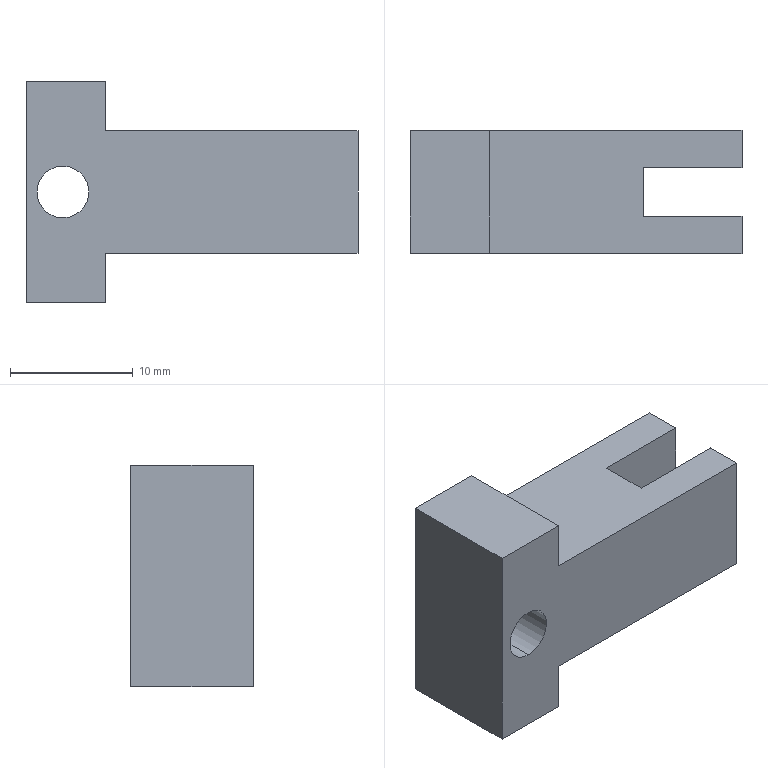Part | SolidWorks | features ICE 7, Extrusion 1, HoleWzd 1, MirrorPattern 1 | 1 solid | 26 faces | box 27 x 10 x 18 mm | volume 2677 mm3 | plane 20 | cylinder 6 | commonest cylinder face diameters 2 x2 2.6 x2 4.2 x2
STEP:
#1=CARTESIAN_POINT('',(-16.,10.,-2.1));
#2=VERTEX_POINT('',#1);
#3=CARTESIAN_POINT('',(-16.,10.,2.1));
#4=VERTEX_POINT('',#3);
#5=CARTESIAN_POINT('',(-16.,10.,0.));
#6=DIRECTION('',(0.,1.,0.));
#7=DIRECTION('',(0.,0.,1.));
#8=AXIS2_PLACEMENT_3D('',#5,#6,#7);
#9=CIRCLE('',#8,2.1);
#10=EDGE_CURVE('',#2,#4,#9,.T.);
#11=ORIENTED_EDGE('',*,*,#10,.T.);
#12=CARTESIAN_POINT('',(-16.,0.,2.1));
#13=VERTEX_POINT('',#12);
#14=CARTESIAN_POINT('',(-16.,0.,2.1));
#15=DIRECTION('',(0.,-1.,0.));
#16=VECTOR('',#15,1000.);
#17=LINE('',#14,#16);
#18=EDGE_CURVE('',#4,#13,#17,.T.);
#19=ORIENTED_EDGE('',*,*,#18,.T.);
#20=CARTESIAN_POINT('',(-16.,0.,-2.1));
#21=VERTEX_POINT('',#20);
#22=CARTESIAN_POINT('',(-16.,0.,0.));
#23=DIRECTION('',(0.,-1.,0.));
#24=DIRECTION('',(0.,0.,-1.));
#25=AXIS2_PLACEMENT_3D('',#22,#23,#24);
#26=CIRCLE('',#25,2.1);
#27=EDGE_CURVE('',#13,#21,#26,.T.);
#28=ORIENTED_EDGE('',*,*,#27,.T.);
#29=CARTESIAN_POINT('',(-16.,0.,-2.1));
#30=DIRECTION('',(0.,-1.,0.));
#31=VECTOR('',#30,1000.);
#32=LINE('',#29,#31);
#33=EDGE_CURVE('',#2,#21,#32,.T.);
#34=ORIENTED_EDGE('',*,*,#33,.F.);
#35=EDGE_LOOP('',(#11,#19,#28,#34));
#36=FACE_OUTER_BOUND('',#35,.T.);
#37=CARTESIAN_POINT('',(-16.,0.,0.));
#38=DIRECTION('',(0.,-1.,0.));
#39=DIRECTION('',(0.,0.,-1.));
#40=AXIS2_PLACEMENT_3D('',#37,#38,#39);
#41=CYLINDRICAL_SURFACE('',#40,2.1);
#42=ADVANCED_FACE('',(#36),#41,.F.);
#43=CARTESIAN_POINT('',(-2.,5.,-1.3));
#44=VERTEX_POINT('',#43);
#45=CARTESIAN_POINT('',(-2.,5.,1.3));
#46=VERTEX_POINT('',#45);
#47=CARTESIAN_POINT('',(-2.,5.,0.));
#48=DIRECTION('',(1.,0.,0.));
#49=DIRECTION('',(0.,0.,-1.));
#50=AXIS2_PLACEMENT_3D('',#47,#48,#49);
#51=CIRCLE('',#50,1.3);
#52=EDGE_CURVE('',#44,#46,#51,.T.);
#53=ORIENTED_EDGE('',*,*,#52,.T.);
#54=CARTESIAN_POINT('',(-1.,5.,1.3));
#55=VERTEX_POINT('',#54);
#56=CARTESIAN_POINT('',(-2.,5.,1.3));
#57=DIRECTION('',(1.,0.,0.));
#58=VECTOR('',#57,1000.);
#59=LINE('',#56,#58);
#60=EDGE_CURVE('',#46,#55,#59,.T.);
#61=ORIENTED_EDGE('',*,*,#60,.T.);
#62=CARTESIAN_POINT('',(-1.,5.,-1.3));
#63=VERTEX_POINT('',#62);
#64=CARTESIAN_POINT('',(-1.,5.,0.));
#65=DIRECTION('',(1.,0.,0.));
#66=DIRECTION('',(0.,0.,-1.));
#67=AXIS2_PLACEMENT_3D('',#64,#65,#66);
#68=CIRCLE('',#67,1.3);
#69=EDGE_CURVE('',#63,#55,#68,.T.);
#70=ORIENTED_EDGE('',*,*,#69,.F.);
#71=CARTESIAN_POINT('',(-2.,5.,-1.3));
#72=DIRECTION('',(1.,0.,0.));
#73=VECTOR('',#72,1000.);
#74=LINE('',#71,#73);
#75=EDGE_CURVE('',#44,#63,#74,.T.);
#76=ORIENTED_EDGE('',*,*,#75,.F.);
#77=EDGE_LOOP('',(#53,#61,#70,#76));
#78=FACE_OUTER_BOUND('',#77,.T.);
#79=CARTESIAN_POINT('',(-2.,5.,0.));
#80=DIRECTION('',(1.,0.,0.));
#81=DIRECTION('',(0.,0.,-1.));
#82=AXIS2_PLACEMENT_3D('',#79,#80,#81);
#83=CYLINDRICAL_SURFACE('',#82,1.3);
#84=ADVANCED_FACE('',(#78),#83,.T.);
#85=CARTESIAN_POINT('',(-2.,5.,-1.));
#86=VERTEX_POINT('',#85);
#87=CARTESIAN_POINT('',(-2.,5.,1.));
#88=VERTEX_POINT('',#87);
#89=CARTESIAN_POINT('',(-2.,5.,0.));
#90=DIRECTION('',(1.,0.,0.));
#91=DIRECTION('',(0.,0.,-1.));
#92=AXIS2_PLACEMENT_3D('',#89,#90,#91);
#93=CIRCLE('',#92,1.);
#94=EDGE_CURVE('',#86,#88,#93,.T.);
#95=ORIENTED_EDGE('',*,*,#94,.F.);
#96=CARTESIAN_POINT('',(-4.,5.,-1.));
#97=VERTEX_POINT('',#96);
#98=CARTESIAN_POINT('',(-1.,5.,-1.));
#99=DIRECTION('',(-1.,0.,0.));
#100=VECTOR('',#99,1000.);
#101=LINE('',#98,#100);
#102=EDGE_CURVE('',#86,#97,#101,.T.);
#103=ORIENTED_EDGE('',*,*,#102,.T.);
#104=CARTESIAN_POINT('',(-4.,5.,1.));
#105=VERTEX_POINT('',#104);
#106=CARTESIAN_POINT('',(-4.,5.,0.));
#107=DIRECTION('',(1.,0.,0.));
#108=DIRECTION('',(0.,0.,-1.));
#109=AXIS2_PLACEMENT_3D('',#106,#107,#108);
#110=CIRCLE('',#109,1.);
#111=EDGE_CURVE('',#97,#105,#110,.T.);
#112=ORIENTED_EDGE('',*,*,#111,.T.);
#113=CARTESIAN_POINT('',(-1.,5.,1.));
#114=DIRECTION('',(-1.,0.,0.));
#115=VECTOR('',#114,1000.);
#116=LINE('',#113,#115);
#117=EDGE_CURVE('',#88,#105,#116,.T.);
#118=ORIENTED_EDGE('',*,*,#117,.F.);
#119=EDGE_LOOP('',(#95,#103,#112,#118));
#120=FACE_OUTER_BOUND('',#119,.T.);
#121=CARTESIAN_POINT('',(-1.,5.,0.));
#122=DIRECTION('',(-1.,0.,0.));
#123=DIRECTION('',(0.,0.,1.));
#124=AXIS2_PLACEMENT_3D('',#121,#122,#123);
#125=CYLINDRICAL_SURFACE('',#124,1.);
#126=ADVANCED_FACE('',(#120),#125,.T.);
#127=ORIENTED_EDGE('',*,*,#102,.F.);
#128=CARTESIAN_POINT('',(-2.,5.,0.));
#129=DIRECTION('',(1.,0.,0.));
#130=DIRECTION('',(0.,0.,-1.));
#131=AXIS2_PLACEMENT_3D('',#128,#129,#130);
#132=CIRCLE('',#131,1.);
#133=EDGE_CURVE('',#88,#86,#132,.T.);
#134=ORIENTED_EDGE('',*,*,#133,.F.);
#135=ORIENTED_EDGE('',*,*,#117,.T.);
#136=CARTESIAN_POINT('',(-4.,5.,0.));
#137=DIRECTION('',(1.,0.,0.));
#138=DIRECTION('',(0.,0.,-1.));
#139=AXIS2_PLACEMENT_3D('',#136,#137,#138);
#140=CIRCLE('',#139,1.);
#141=EDGE_CURVE('',#105,#97,#140,.T.);
#142=ORIENTED_EDGE('',*,*,#141,.T.);
#143=EDGE_LOOP('',(#127,#134,#135,#142));
#144=FACE_OUTER_BOUND('',#143,.T.);
#145=CARTESIAN_POINT('',(-1.,5.,0.));
#146=DIRECTION('',(-1.,0.,0.));
#147=DIRECTION('',(0.,0.,1.));
#148=AXIS2_PLACEMENT_3D('',#145,#146,#147);
#149=CYLINDRICAL_SURFACE('',#148,1.);
#150=ADVANCED_FACE('',(#144),#149,.T.);
#151=CARTESIAN_POINT('',(0.,3.,5.));
#152=VERTEX_POINT('',#151);
#153=CARTESIAN_POINT('',(0.,3.,3.));
#154=VERTEX_POINT('',#153);
#155=CARTESIAN_POINT('',(0.,3.,5.));
#156=DIRECTION('',(0.,0.,-1.));
#157=VECTOR('',#156,1000.);
#158=LINE('',#155,#157);
#159=EDGE_CURVE('',#152,#154,#158,.T.);
#160=ORIENTED_EDGE('',*,*,#159,.T.);
#161=CARTESIAN_POINT('',(0.,7.,3.));
#162=VERTEX_POINT('',#161);
#163=CARTESIAN_POINT('',(0.,3.,3.));
#164=DIRECTION('',(0.,-1.,0.));
#165=VECTOR('',#164,1000.);
#166=LINE('',#163,#165);
#167=EDGE_CURVE('',#162,#154,#166,.T.);
#168=ORIENTED_EDGE('',*,*,#167,.F.);
#169=CARTESIAN_POINT('',(0.,7.,5.));
#170=VERTEX_POINT('',#169);
#171=CARTESIAN_POINT('',(0.,7.,5.));
#172=DIRECTION('',(0.,0.,-1.));
#173=VECTOR('',#172,1000.);
#174=LINE('',#171,#173);
#175=EDGE_CURVE('',#170,#162,#174,.T.);
#176=ORIENTED_EDGE('',*,*,#175,.F.);
#177=CARTESIAN_POINT('',(0.,3.,5.));
#178=DIRECTION('',(0.,1.,0.));
#179=VECTOR('',#178,1000.);
#180=LINE('',#177,#179);
#181=EDGE_CURVE('',#152,#170,#180,.T.);
#182=ORIENTED_EDGE('',*,*,#181,.F.);
#183=EDGE_LOOP('',(#160,#168,#176,#182));
#184=FACE_OUTER_BOUND('',#183,.T.);
#185=CARTESIAN_POINT('',(0.,3.,5.));
#186=DIRECTION('',(-1.,0.,0.));
#187=DIRECTION('',(0.,0.,1.));
#188=AXIS2_PLACEMENT_3D('',#185,#186,#187);
#189=PLANE('',#188);
#190=ADVANCED_FACE('',(#184),#189,.F.);
#191=CARTESIAN_POINT('',(-12.5,10.,-5.));
#192=VERTEX_POINT('',#191);
#193=CARTESIAN_POINT('',(-12.5,0.,-5.));
#194=VERTEX_POINT('',#193);
#195=CARTESIAN_POINT('',(-12.5,0.,-5.));
#196=DIRECTION('',(0.,-1.,0.));
#197=VECTOR('',#196,1000.);
#198=LINE('',#195,#197);
#199=EDGE_CURVE('',#192,#194,#198,.T.);
#200=ORIENTED_EDGE('',*,*,#199,.F.);
#201=CARTESIAN_POINT('',(8.,10.,-5.));
#202=VERTEX_POINT('',#201);
#203=CARTESIAN_POINT('',(8.,10.,-5.));
#204=DIRECTION('',(-1.,0.,0.));
#205=VECTOR('',#204,1000.);
#206=LINE('',#203,#205);
#207=EDGE_CURVE('',#202,#192,#206,.T.);
#208=ORIENTED_EDGE('',*,*,#207,.F.);
#209=CARTESIAN_POINT('',(8.,7.,-5.));
#210=VERTEX_POINT('',#209);
#211=CARTESIAN_POINT('',(8.,10.,-5.));
#212=DIRECTION('',(0.,-1.,0.));
#213=VECTOR('',#212,1000.);
#214=LINE('',#211,#213);
#215=EDGE_CURVE('',#202,#210,#214,.T.);
#216=ORIENTED_EDGE('',*,*,#215,.T.);
#217=CARTESIAN_POINT('',(0.,7.,-5.));
#218=VERTEX_POINT('',#217);
#219=CARTESIAN_POINT('',(16.,7.,-5.));
#220=DIRECTION('',(1.,0.,0.));
#221=VECTOR('',#220,1000.);
#222=LINE('',#219,#221);
#223=EDGE_CURVE('',#218,#210,#222,.T.);
#224=ORIENTED_EDGE('',*,*,#223,.F.);
#225=CARTESIAN_POINT('',(0.,3.,-5.));
#226=VERTEX_POINT('',#225);
#227=CARTESIAN_POINT('',(0.,3.,-5.));
#228=DIRECTION('',(0.,1.,0.));
#229=VECTOR('',#228,1000.);
#230=LINE('',#227,#229);
#231=EDGE_CURVE('',#226,#218,#230,.T.);
#232=ORIENTED_EDGE('',*,*,#231,.F.);
#233=CARTESIAN_POINT('',(8.,3.,-5.));
#234=VERTEX_POINT('',#233);
#235=CARTESIAN_POINT('',(8.,3.,-5.));
#236=DIRECTION('',(1.,0.,0.));
#237=VECTOR('',#236,1000.);
#238=LINE('',#235,#237);
#239=EDGE_CURVE('',#226,#234,#238,.T.);
#240=ORIENTED_EDGE('',*,*,#239,.T.);
#241=CARTESIAN_POINT('',(8.,0.,-5.));
#242=VERTEX_POINT('',#241);
#243=CARTESIAN_POINT('',(8.,10.,-5.));
#244=DIRECTION('',(0.,-1.,0.));
#245=VECTOR('',#244,1000.);
#246=LINE('',#243,#245);
#247=EDGE_CURVE('',#234,#242,#246,.T.);
#248=ORIENTED_EDGE('',*,*,#247,.T.);
#249=CARTESIAN_POINT('',(8.,0.,-5.));
#250=DIRECTION('',(-1.,0.,0.));
#251=VECTOR('',#250,1000.);
#252=LINE('',#249,#251);
#253=EDGE_CURVE('',#242,#194,#252,.T.);
#254=ORIENTED_EDGE('',*,*,#253,.T.);
#255=EDGE_LOOP('',(#200,#208,#216,#224,#232,#240,#248,#254));
#256=FACE_OUTER_BOUND('',#255,.T.);
#257=CARTESIAN_POINT('',(8.,10.,-5.));
#258=DIRECTION('',(0.,0.,1.));
#259=DIRECTION('',(1.,0.,0.));
#260=AXIS2_PLACEMENT_3D('',#257,#258,#259);
#261=PLANE('',#260);
#262=ADVANCED_FACE('',(#256),#261,.F.);
#263=ORIENTED_EDGE('',*,*,#247,.F.);
#264=CARTESIAN_POINT('',(8.,3.,5.));
#265=VERTEX_POINT('',#264);
#266=CARTESIAN_POINT('',(8.,3.,5.));
#267=DIRECTION('',(0.,0.,1.));
#268=VECTOR('',#267,1000.);
#269=LINE('',#266,#268);
#270=EDGE_CURVE('',#234,#265,#269,.T.);
#271=ORIENTED_EDGE('',*,*,#270,.T.);
#272=CARTESIAN_POINT('',(8.,0.,5.));
#273=VERTEX_POINT('',#272);
#274=CARTESIAN_POINT('',(8.,10.,5.));
#275=DIRECTION('',(0.,-1.,0.));
#276=VECTOR('',#275,1000.);
#277=LINE('',#274,#276);
#278=EDGE_CURVE('',#265,#273,#277,.T.);
#279=ORIENTED_EDGE('',*,*,#278,.T.);
#280=CARTESIAN_POINT('',(8.,0.,5.));
#281=DIRECTION('',(0.,0.,-1.));
#282=VECTOR('',#281,1000.);
#283=LINE('',#280,#282);
#284=EDGE_CURVE('',#273,#242,#283,.T.);
#285=ORIENTED_EDGE('',*,*,#284,.T.);
#286=EDGE_LOOP('',(#263,#271,#279,#285));
#287=FACE_OUTER_BOUND('',#286,.T.);
#288=CARTESIAN_POINT('',(8.,10.,5.));
#289=DIRECTION('',(-1.,0.,0.));
#290=DIRECTION('',(0.,0.,1.));
#291=AXIS2_PLACEMENT_3D('',#288,#289,#290);
#292=PLANE('',#291);
#293=ADVANCED_FACE('',(#287),#292,.F.);
#294=CARTESIAN_POINT('',(-12.5,10.,5.));
#295=VERTEX_POINT('',#294);
#296=CARTESIAN_POINT('',(8.,10.,5.));
#297=VERTEX_POINT('',#296);
#298=CARTESIAN_POINT('',(8.,10.,5.));
#299=DIRECTION('',(1.,0.,0.));
#300=VECTOR('',#299,1000.);
#301=LINE('',#298,#300);
#302=EDGE_CURVE('',#295,#297,#301,.T.);
#303=ORIENTED_EDGE('',*,*,#302,.F.);
#304=CARTESIAN_POINT('',(-12.5,0.,5.));
#305=VERTEX_POINT('',#304);
#306=CARTESIAN_POINT('',(-12.5,0.,5.));
#307=DIRECTION('',(0.,-1.,0.));
#308=VECTOR('',#307,1000.);
#309=LINE('',#306,#308);
#310=EDGE_CURVE('',#295,#305,#309,.T.);
#311=ORIENTED_EDGE('',*,*,#310,.T.);
#312=CARTESIAN_POINT('',(8.,0.,5.));
#313=DIRECTION('',(1.,0.,0.));
#314=VECTOR('',#313,1000.);
#315=LINE('',#312,#314);
#316=EDGE_CURVE('',#305,#273,#315,.T.);
#317=ORIENTED_EDGE('',*,*,#316,.T.);
#318=ORIENTED_EDGE('',*,*,#278,.F.);
#319=CARTESIAN_POINT('',(16.,3.,5.));
#320=DIRECTION('',(-1.,0.,0.));
#321=VECTOR('',#320,1000.);
#322=LINE('',#319,#321);
#323=EDGE_CURVE('',#265,#152,#322,.T.);
#324=ORIENTED_EDGE('',*,*,#323,.T.);
#325=ORIENTED_EDGE('',*,*,#181,.T.);
#326=CARTESIAN_POINT('',(8.,7.,5.));
#327=VERTEX_POINT('',#326);
#328=CARTESIAN_POINT('',(16.,7.,5.));
#329=DIRECTION('',(1.,0.,0.));
#330=VECTOR('',#329,1000.);
#331=LINE('',#328,#330);
#332=EDGE_CURVE('',#170,#327,#331,.T.);
#333=ORIENTED_EDGE('',*,*,#332,.T.);
#334=CARTESIAN_POINT('',(8.,10.,5.));
#335=DIRECTION('',(0.,-1.,0.));
#336=VECTOR('',#335,1000.);
#337=LINE('',#334,#336);
#338=EDGE_CURVE('',#297,#327,#337,.T.);
#339=ORIENTED_EDGE('',*,*,#338,.F.);
#340=EDGE_LOOP('',(#303,#311,#317,#318,#324,#325,#333,#339));
#341=FACE_OUTER_BOUND('',#340,.T.);
#342=CARTESIAN_POINT('',(8.,10.,5.));
#343=DIRECTION('',(0.,0.,-1.));
#344=DIRECTION('',(-1.,0.,0.));
#345=AXIS2_PLACEMENT_3D('',#342,#343,#344);
#346=PLANE('',#345);
#347=ADVANCED_FACE('',(#341),#346,.F.);
#348=ORIENTED_EDGE('',*,*,#338,.T.);
#349=CARTESIAN_POINT('',(8.,7.,5.));
#350=DIRECTION('',(0.,0.,-1.));
#351=VECTOR('',#350,1000.);
#352=LINE('',#349,#351);
#353=EDGE_CURVE('',#327,#210,#352,.T.);
#354=ORIENTED_EDGE('',*,*,#353,.T.);
#355=ORIENTED_EDGE('',*,*,#215,.F.);
#356=CARTESIAN_POINT('',(8.,10.,5.));
#357=DIRECTION('',(0.,0.,-1.));
#358=VECTOR('',#357,1000.);
#359=LINE('',#356,#358);
#360=EDGE_CURVE('',#297,#202,#359,.T.);
#361=ORIENTED_EDGE('',*,*,#360,.F.);
#362=EDGE_LOOP('',(#348,#354,#355,#361));
#363=FACE_OUTER_BOUND('',#362,.T.);
#364=CARTESIAN_POINT('',(8.,10.,5.));
#365=DIRECTION('',(-1.,0.,0.));
#366=DIRECTION('',(0.,0.,1.));
#367=AXIS2_PLACEMENT_3D('',#364,#365,#366);
#368=PLANE('',#367);
#369=ADVANCED_FACE('',(#363),#368,.F.);
#370=ORIENTED_EDGE('',*,*,#10,.F.);
#371=CARTESIAN_POINT('',(-16.,10.,0.));
#372=DIRECTION('',(0.,1.,0.));
#373=DIRECTION('',(0.,0.,1.));
#374=AXIS2_PLACEMENT_3D('',#371,#372,#373);
#375=CIRCLE('',#374,2.1);
#376=EDGE_CURVE('',#4,#2,#375,.T.);
#377=ORIENTED_EDGE('',*,*,#376,.F.);
#378=EDGE_LOOP('',(#370,#377));
#379=FACE_BOUND('',#378,.T.);
#380=ORIENTED_EDGE('',*,*,#207,.T.);
#381=CARTESIAN_POINT('',(-12.5,10.,-9.));
#382=VERTEX_POINT('',#381);
#383=CARTESIAN_POINT('',(-12.5,10.,-9.));
#384=DIRECTION('',(0.,0.,1.));
#385=VECTOR('',#384,1000.);
#386=LINE('',#383,#385);
#387=EDGE_CURVE('',#382,#192,#386,.T.);
#388=ORIENTED_EDGE('',*,*,#387,.F.);
#389=CARTESIAN_POINT('',(-19.,10.,-9.));
#390=VERTEX_POINT('',#389);
#391=CARTESIAN_POINT('',(-15.,10.,-9.));
#392=DIRECTION('',(1.,0.,0.));
#393=VECTOR('',#392,1000.);
#394=LINE('',#391,#393);
#395=EDGE_CURVE('',#390,#382,#394,.T.);
#396=ORIENTED_EDGE('',*,*,#395,.F.);
#397=CARTESIAN_POINT('',(-19.,10.,9.));
#398=VERTEX_POINT('',#397);
#399=CARTESIAN_POINT('',(-19.,10.,-9.));
#400=DIRECTION('',(0.,0.,-1.));
#401=VECTOR('',#400,1000.);
#402=LINE('',#399,#401);
#403=EDGE_CURVE('',#398,#390,#402,.T.);
#404=ORIENTED_EDGE('',*,*,#403,.F.);
#405=CARTESIAN_POINT('',(-12.5,10.,9.));
#406=VERTEX_POINT('',#405);
#407=CARTESIAN_POINT('',(-15.,10.,9.));
#408=DIRECTION('',(1.,0.,0.));
#409=VECTOR('',#408,1000.);
#410=LINE('',#407,#409);
#411=EDGE_CURVE('',#398,#406,#410,.T.);
#412=ORIENTED_EDGE('',*,*,#411,.T.);
#413=CARTESIAN_POINT('',(-12.5,10.,9.));
#414=DIRECTION('',(0.,0.,-1.));
#415=VECTOR('',#414,1000.);
#416=LINE('',#413,#415);
#417=EDGE_CURVE('',#406,#295,#416,.T.);
#418=ORIENTED_EDGE('',*,*,#417,.T.);
#419=ORIENTED_EDGE('',*,*,#302,.T.);
#420=ORIENTED_EDGE('',*,*,#360,.T.);
#421=EDGE_LOOP('',(#380,#388,#396,#404,#412,#418,#419,#420));
#422=FACE_OUTER_BOUND('',#421,.T.);
#423=CARTESIAN_POINT('',(0.,10.,0.));
#424=DIRECTION('',(0.,1.,0.));
#425=DIRECTION('',(0.,0.,1.));
#426=AXIS2_PLACEMENT_3D('',#423,#424,#425);
#427=PLANE('',#426);
#428=ADVANCED_FACE('',(#379,#422),#427,.T.);
#429=CARTESIAN_POINT('',(-16.,0.,0.));
#430=DIRECTION('',(0.,-1.,0.));
#431=DIRECTION('',(0.,0.,-1.));
#432=AXIS2_PLACEMENT_3D('',#429,#430,#431);
#433=CIRCLE('',#432,2.1);
#434=EDGE_CURVE('',#21,#13,#433,.T.);
#435=ORIENTED_EDGE('',*,*,#434,.F.);
#436=ORIENTED_EDGE('',*,*,#27,.F.);
#437=EDGE_LOOP('',(#435,#436));
#438=FACE_BOUND('',#437,.T.);
#439=ORIENTED_EDGE('',*,*,#316,.F.);
#440=CARTESIAN_POINT('',(-12.5,0.,9.));
#441=VERTEX_POINT('',#440);
#442=CARTESIAN_POINT('',(-12.5,0.,9.));
#443=DIRECTION('',(0.,0.,-1.));
#444=VECTOR('',#443,1000.);
#445=LINE('',#442,#444);
#446=EDGE_CURVE('',#441,#305,#445,.T.);
#447=ORIENTED_EDGE('',*,*,#446,.F.);
#448=CARTESIAN_POINT('',(-19.,0.,9.));
#449=VERTEX_POINT('',#448);
#450=CARTESIAN_POINT('',(-15.,0.,9.));
#451=DIRECTION('',(-1.,0.,0.));
#452=VECTOR('',#451,1000.);
#453=LINE('',#450,#452);
#454=EDGE_CURVE('',#441,#449,#453,.T.);
#455=ORIENTED_EDGE('',*,*,#454,.T.);
#456=CARTESIAN_POINT('',(-19.,0.,-9.));
#457=VERTEX_POINT('',#456);
#458=CARTESIAN_POINT('',(-19.,0.,-9.));
#459=DIRECTION('',(0.,0.,1.));
#460=VECTOR('',#459,1000.);
#461=LINE('',#458,#460);
#462=EDGE_CURVE('',#457,#449,#461,.T.);
#463=ORIENTED_EDGE('',*,*,#462,.F.);
#464=CARTESIAN_POINT('',(-12.5,0.,-9.));
#465=VERTEX_POINT('',#464);
#466=CARTESIAN_POINT('',(-15.,0.,-9.));
#467=DIRECTION('',(-1.,0.,0.));
#468=VECTOR('',#467,1000.);
#469=LINE('',#466,#468);
#470=EDGE_CURVE('',#465,#457,#469,.T.);
#471=ORIENTED_EDGE('',*,*,#470,.F.);
#472=CARTESIAN_POINT('',(-12.5,0.,-9.));
#473=DIRECTION('',(0.,0.,1.));
#474=VECTOR('',#473,1000.);
#475=LINE('',#472,#474);
#476=EDGE_CURVE('',#465,#194,#475,.T.);
#477=ORIENTED_EDGE('',*,*,#476,.T.);
#478=ORIENTED_EDGE('',*,*,#253,.F.);
#479=ORIENTED_EDGE('',*,*,#284,.F.);
#480=EDGE_LOOP('',(#439,#447,#455,#463,#471,#477,#478,#479));
#481=FACE_OUTER_BOUND('',#480,.T.);
#482=CARTESIAN_POINT('',(0.,0.,0.));
#483=DIRECTION('',(0.,1.,0.));
#484=DIRECTION('',(0.,0.,1.));
#485=AXIS2_PLACEMENT_3D('',#482,#483,#484);
#486=PLANE('',#485);
#487=ADVANCED_FACE('',(#438,#481),#486,.F.);
#488=ORIENTED_EDGE('',*,*,#239,.F.);
#489=CARTESIAN_POINT('',(0.,3.,-3.));
#490=VERTEX_POINT('',#489);
#491=CARTESIAN_POINT('',(0.,3.,5.));
#492=DIRECTION('',(0.,0.,-1.));
#493=VECTOR('',#492,1000.);
#494=LINE('',#491,#493);
#495=EDGE_CURVE('',#490,#226,#494,.T.);
#496=ORIENTED_EDGE('',*,*,#495,.F.);
#497=CARTESIAN_POINT('',(-4.,3.,-3.));
#498=VERTEX_POINT('',#497);
#499=CARTESIAN_POINT('',(-4.,3.,-3.));
#500=DIRECTION('',(1.,0.,0.));
#501=VECTOR('',#500,1000.);
#502=LINE('',#499,#501);
#503=EDGE_CURVE('',#498,#490,#502,.T.);
#504=ORIENTED_EDGE('',*,*,#503,.F.);
#505=CARTESIAN_POINT('',(-4.,3.,3.));
#506=VERTEX_POINT('',#505);
#507=CARTESIAN_POINT('',(-4.,3.,-3.));
#508=DIRECTION('',(0.,0.,-1.));
#509=VECTOR('',#508,1000.);
#510=LINE('',#507,#509);
#511=EDGE_CURVE('',#506,#498,#510,.T.);
#512=ORIENTED_EDGE('',*,*,#511,.F.);
#513=CARTESIAN_POINT('',(-4.,3.,3.));
#514=DIRECTION('',(1.,0.,0.));
#515=VECTOR('',#514,1000.);
#516=LINE('',#513,#515);
#517=EDGE_CURVE('',#506,#154,#516,.T.);
#518=ORIENTED_EDGE('',*,*,#517,.T.);
#519=ORIENTED_EDGE('',*,*,#159,.F.);
#520=ORIENTED_EDGE('',*,*,#323,.F.);
#521=ORIENTED_EDGE('',*,*,#270,.F.);
#522=EDGE_LOOP('',(#488,#496,#504,#512,#518,#519,#520,#521));
#523=FACE_OUTER_BOUND('',#522,.T.);
#524=CARTESIAN_POINT('',(16.,3.,5.));
#525=DIRECTION('',(0.,-1.,0.));
#526=DIRECTION('',(0.,0.,-1.));
#527=AXIS2_PLACEMENT_3D('',#524,#525,#526);
#528=PLANE('',#527);
#529=ADVANCED_FACE('',(#523),#528,.F.);
#530=ORIENTED_EDGE('',*,*,#332,.F.);
#531=ORIENTED_EDGE('',*,*,#175,.T.);
#532=CARTESIAN_POINT('',(-4.,7.,3.));
#533=VERTEX_POINT('',#532);
#534=CARTESIAN_POINT('',(-4.,7.,3.));
#535=DIRECTION('',(1.,0.,0.));
#536=VECTOR('',#535,1000.);
#537=LINE('',#534,#536);
#538=EDGE_CURVE('',#533,#162,#537,.T.);
#539=ORIENTED_EDGE('',*,*,#538,.F.);
#540=CARTESIAN_POINT('',(-4.,7.,-3.));
#541=VERTEX_POINT('',#540);
#542=CARTESIAN_POINT('',(-4.,7.,-3.));
#543=DIRECTION('',(0.,0.,1.));
#544=VECTOR('',#543,1000.);
#545=LINE('',#542,#544);
#546=EDGE_CURVE('',#541,#533,#545,.T.);
#547=ORIENTED_EDGE('',*,*,#546,.F.);
#548=CARTESIAN_POINT('',(0.,7.,-3.));
#549=VERTEX_POINT('',#548);
#550=CARTESIAN_POINT('',(-4.,7.,-3.));
#551=DIRECTION('',(1.,0.,0.));
#552=VECTOR('',#551,1000.);
#553=LINE('',#550,#552);
#554=EDGE_CURVE('',#541,#549,#553,.T.);
#555=ORIENTED_EDGE('',*,*,#554,.T.);
#556=CARTESIAN_POINT('',(0.,7.,5.));
#557=DIRECTION('',(0.,0.,-1.));
#558=VECTOR('',#557,1000.);
#559=LINE('',#556,#558);
#560=EDGE_CURVE('',#549,#218,#559,.T.);
#561=ORIENTED_EDGE('',*,*,#560,.T.);
#562=ORIENTED_EDGE('',*,*,#223,.T.);
#563=ORIENTED_EDGE('',*,*,#353,.F.);
#564=EDGE_LOOP('',(#530,#531,#539,#547,#555,#561,#562,#563));
#565=FACE_OUTER_BOUND('',#564,.T.);
#566=CARTESIAN_POINT('',(16.,7.,5.));
#567=DIRECTION('',(0.,1.,0.));
#568=DIRECTION('',(0.,0.,1.));
#569=AXIS2_PLACEMENT_3D('',#566,#567,#568);
#570=PLANE('',#569);
#571=ADVANCED_FACE('',(#565),#570,.F.);
#572=ORIENTED_EDGE('',*,*,#560,.F.);
#573=CARTESIAN_POINT('',(0.,3.,-3.));
#574=DIRECTION('',(0.,1.,0.));
#575=VECTOR('',#574,1000.);
#576=LINE('',#573,#575);
#577=EDGE_CURVE('',#490,#549,#576,.T.);
#578=ORIENTED_EDGE('',*,*,#577,.F.);
#579=ORIENTED_EDGE('',*,*,#495,.T.);
#580=ORIENTED_EDGE('',*,*,#231,.T.);
#581=EDGE_LOOP('',(#572,#578,#579,#580));
#582=FACE_OUTER_BOUND('',#581,.T.);
#583=CARTESIAN_POINT('',(0.,3.,5.));
#584=DIRECTION('',(-1.,0.,0.));
#585=DIRECTION('',(0.,0.,1.));
#586=AXIS2_PLACEMENT_3D('',#583,#584,#585);
#587=PLANE('',#586);
#588=ADVANCED_FACE('',(#582),#587,.F.);
#589=ORIENTED_EDGE('',*,*,#199,.T.);
#590=ORIENTED_EDGE('',*,*,#476,.F.);
#591=CARTESIAN_POINT('',(-12.5,0.,-9.));
#592=DIRECTION('',(0.,-1.,0.));
#593=VECTOR('',#592,1000.);
#594=LINE('',#591,#593);
#595=EDGE_CURVE('',#382,#465,#594,.T.);
#596=ORIENTED_EDGE('',*,*,#595,.F.);
#597=ORIENTED_EDGE('',*,*,#387,.T.);
#598=EDGE_LOOP('',(#589,#590,#596,#597));
#599=FACE_OUTER_BOUND('',#598,.T.);
#600=CARTESIAN_POINT('',(-12.5,0.,-9.));
#601=DIRECTION('',(-1.,0.,0.));
#602=DIRECTION('',(0.,-1.,0.));
#603=AXIS2_PLACEMENT_3D('',#600,#601,#602);
#604=PLANE('',#603);
#605=ADVANCED_FACE('',(#599),#604,.F.);
#606=ORIENTED_EDGE('',*,*,#470,.T.);
#607=CARTESIAN_POINT('',(-19.,10.,-9.));
#608=DIRECTION('',(0.,-1.,0.));
#609=VECTOR('',#608,1000.);
#610=LINE('',#607,#609);
#611=EDGE_CURVE('',#390,#457,#610,.T.);
#612=ORIENTED_EDGE('',*,*,#611,.F.);
#613=ORIENTED_EDGE('',*,*,#395,.T.);
#614=ORIENTED_EDGE('',*,*,#595,.T.);
#615=EDGE_LOOP('',(#606,#612,#613,#614));
#616=FACE_OUTER_BOUND('',#615,.T.);
#617=CARTESIAN_POINT('',(0.,0.,-9.));
#618=DIRECTION('',(0.,0.,-1.));
#619=DIRECTION('',(-1.,0.,0.));
#620=AXIS2_PLACEMENT_3D('',#617,#618,#619);
#621=PLANE('',#620);
#622=ADVANCED_FACE('',(#616),#621,.T.);
#623=ORIENTED_EDGE('',*,*,#310,.F.);
#624=ORIENTED_EDGE('',*,*,#417,.F.);
#625=CARTESIAN_POINT('',(-12.5,0.,9.));
#626=DIRECTION('',(0.,-1.,0.));
#627=VECTOR('',#626,1000.);
#628=LINE('',#625,#627);
#629=EDGE_CURVE('',#406,#441,#628,.T.);
#630=ORIENTED_EDGE('',*,*,#629,.T.);
#631=ORIENTED_EDGE('',*,*,#446,.T.);
#632=EDGE_LOOP('',(#623,#624,#630,#631));
#633=FACE_OUTER_BOUND('',#632,.T.);
#634=CARTESIAN_POINT('',(-12.5,0.,9.));
#635=DIRECTION('',(1.,0.,0.));
#636=DIRECTION('',(0.,1.,0.));
#637=AXIS2_PLACEMENT_3D('',#634,#635,#636);
#638=PLANE('',#637);
#639=ADVANCED_FACE('',(#633),#638,.T.);
#640=ORIENTED_EDGE('',*,*,#411,.F.);
#641=CARTESIAN_POINT('',(-19.,10.,9.));
#642=DIRECTION('',(0.,1.,0.));
#643=VECTOR('',#642,1000.);
#644=LINE('',#641,#643);
#645=EDGE_CURVE('',#449,#398,#644,.T.);
#646=ORIENTED_EDGE('',*,*,#645,.F.);
#647=ORIENTED_EDGE('',*,*,#454,.F.);
#648=ORIENTED_EDGE('',*,*,#629,.F.);
#649=EDGE_LOOP('',(#640,#646,#647,#648));
#650=FACE_OUTER_BOUND('',#649,.T.);
#651=CARTESIAN_POINT('',(0.,0.,9.));
#652=DIRECTION('',(0.,0.,1.));
#653=DIRECTION('',(-1.,0.,0.));
#654=AXIS2_PLACEMENT_3D('',#651,#652,#653);
#655=PLANE('',#654);
#656=ADVANCED_FACE('',(#650),#655,.T.);
#657=ORIENTED_EDGE('',*,*,#167,.T.);
#658=ORIENTED_EDGE('',*,*,#517,.F.);
#659=CARTESIAN_POINT('',(-4.,3.,3.));
#660=DIRECTION('',(0.,-1.,0.));
#661=VECTOR('',#660,1000.);
#662=LINE('',#659,#661);
#663=EDGE_CURVE('',#533,#506,#662,.T.);
#664=ORIENTED_EDGE('',*,*,#663,.F.);
#665=ORIENTED_EDGE('',*,*,#538,.T.);
#666=EDGE_LOOP('',(#657,#658,#664,#665));
#667=FACE_OUTER_BOUND('',#666,.T.);
#668=CARTESIAN_POINT('',(-4.,3.,3.));
#669=DIRECTION('',(0.,0.,1.));
#670=DIRECTION('',(1.,0.,0.));
#671=AXIS2_PLACEMENT_3D('',#668,#669,#670);
#672=PLANE('',#671);
#673=ADVANCED_FACE('',(#667),#672,.F.);
#674=ORIENTED_EDGE('',*,*,#577,.T.);
#675=ORIENTED_EDGE('',*,*,#554,.F.);
#676=CARTESIAN_POINT('',(-4.,3.,-3.));
#677=DIRECTION('',(0.,1.,0.));
#678=VECTOR('',#677,1000.);
#679=LINE('',#676,#678);
#680=EDGE_CURVE('',#498,#541,#679,.T.);
#681=ORIENTED_EDGE('',*,*,#680,.F.);
#682=ORIENTED_EDGE('',*,*,#503,.T.);
#683=EDGE_LOOP('',(#674,#675,#681,#682));
#684=FACE_OUTER_BOUND('',#683,.T.);
#685=CARTESIAN_POINT('',(-4.,3.,-3.));
#686=DIRECTION('',(0.,0.,-1.));
#687=DIRECTION('',(-1.,0.,0.));
#688=AXIS2_PLACEMENT_3D('',#685,#686,#687);
#689=PLANE('',#688);
#690=ADVANCED_FACE('',(#684),#689,.F.);
#691=ORIENTED_EDGE('',*,*,#141,.F.);
#692=ORIENTED_EDGE('',*,*,#111,.F.);
#693=EDGE_LOOP('',(#691,#692));
#694=FACE_BOUND('',#693,.T.);
#695=ORIENTED_EDGE('',*,*,#663,.T.);
#696=ORIENTED_EDGE('',*,*,#511,.T.);
#697=ORIENTED_EDGE('',*,*,#680,.T.);
#698=ORIENTED_EDGE('',*,*,#546,.T.);
#699=EDGE_LOOP('',(#695,#696,#697,#698));
#700=FACE_OUTER_BOUND('',#699,.T.);
#701=CARTESIAN_POINT('',(-4.,0.,0.));
#702=DIRECTION('',(1.,0.,0.));
#703=DIRECTION('',(0.,0.,-1.));
#704=AXIS2_PLACEMENT_3D('',#701,#702,#703);
#705=PLANE('',#704);
#706=ADVANCED_FACE('',(#694,#700),#705,.T.);
#707=ORIENTED_EDGE('',*,*,#60,.F.);
#708=CARTESIAN_POINT('',(-2.,5.,0.));
#709=DIRECTION('',(1.,0.,0.));
#710=DIRECTION('',(0.,0.,-1.));
#711=AXIS2_PLACEMENT_3D('',#708,#709,#710);
#712=CIRCLE('',#711,1.3);
#713=EDGE_CURVE('',#46,#44,#712,.T.);
#714=ORIENTED_EDGE('',*,*,#713,.T.);
#715=ORIENTED_EDGE('',*,*,#75,.T.);
#716=CARTESIAN_POINT('',(-1.,5.,0.));
#717=DIRECTION('',(1.,0.,0.));
#718=DIRECTION('',(0.,0.,-1.));
#719=AXIS2_PLACEMENT_3D('',#716,#717,#718);
#720=CIRCLE('',#719,1.3);
#721=EDGE_CURVE('',#55,#63,#720,.T.);
#722=ORIENTED_EDGE('',*,*,#721,.F.);
#723=EDGE_LOOP('',(#707,#714,#715,#722));
#724=FACE_OUTER_BOUND('',#723,.T.);
#725=CARTESIAN_POINT('',(-2.,5.,0.));
#726=DIRECTION('',(1.,0.,0.));
#727=DIRECTION('',(0.,0.,-1.));
#728=AXIS2_PLACEMENT_3D('',#725,#726,#727);
#729=CYLINDRICAL_SURFACE('',#728,1.3);
#730=ADVANCED_FACE('',(#724),#729,.T.);
#731=ORIENTED_EDGE('',*,*,#133,.T.);
#732=ORIENTED_EDGE('',*,*,#94,.T.);
#733=EDGE_LOOP('',(#731,#732));
#734=FACE_BOUND('',#733,.T.);
#735=ORIENTED_EDGE('',*,*,#52,.F.);
#736=ORIENTED_EDGE('',*,*,#713,.F.);
#737=EDGE_LOOP('',(#735,#736));
#738=FACE_OUTER_BOUND('',#737,.T.);
#739=CARTESIAN_POINT('',(-2.,5.,0.));
#740=DIRECTION('',(1.,0.,0.));
#741=DIRECTION('',(0.,0.,-1.));
#742=AXIS2_PLACEMENT_3D('',#739,#740,#741);
#743=PLANE('',#742);
#744=ADVANCED_FACE('',(#734,#738),#743,.F.);
#745=ORIENTED_EDGE('',*,*,#69,.T.);
#746=ORIENTED_EDGE('',*,*,#721,.T.);
#747=EDGE_LOOP('',(#745,#746));
#748=FACE_OUTER_BOUND('',#747,.T.);
#749=CARTESIAN_POINT('',(-1.,5.,0.));
#750=DIRECTION('',(1.,0.,0.));
#751=DIRECTION('',(0.,0.,-1.));
#752=AXIS2_PLACEMENT_3D('',#749,#750,#751);
#753=PLANE('',#752);
#754=ADVANCED_FACE('',(#748),#753,.T.);
#755=ORIENTED_EDGE('',*,*,#611,.T.);
#756=ORIENTED_EDGE('',*,*,#462,.T.);
#757=ORIENTED_EDGE('',*,*,#645,.T.);
#758=ORIENTED_EDGE('',*,*,#403,.T.);
#759=EDGE_LOOP('',(#755,#756,#757,#758));
#760=FACE_OUTER_BOUND('',#759,.T.);
#761=CARTESIAN_POINT('',(-19.,0.,0.));
#762=DIRECTION('',(-1.,0.,0.));
#763=DIRECTION('',(0.,0.,1.));
#764=AXIS2_PLACEMENT_3D('',#761,#762,#763);
#765=PLANE('',#764);
#766=ADVANCED_FACE('',(#760),#765,.T.);
#767=ORIENTED_EDGE('',*,*,#18,.F.);
#768=ORIENTED_EDGE('',*,*,#376,.T.);
#769=ORIENTED_EDGE('',*,*,#33,.T.);
#770=ORIENTED_EDGE('',*,*,#434,.T.);
#771=EDGE_LOOP('',(#767,#768,#769,#770));
#772=FACE_OUTER_BOUND('',#771,.T.);
#773=CARTESIAN_POINT('',(-16.,0.,0.));
#774=DIRECTION('',(0.,-1.,0.));
#775=DIRECTION('',(0.,0.,-1.));
#776=AXIS2_PLACEMENT_3D('',#773,#774,#775);
#777=CYLINDRICAL_SURFACE('',#776,2.1);
#778=ADVANCED_FACE('',(#772),#777,.F.);
#779=CLOSED_SHELL('',(#42,#84,#126,#150,#190,#262,#293,#347,#369,#428,#487,#529,#571,#588,#605,#622,#639,#656,#673,#690,#706,#730,#744,#754,#766,#778));
#780=MANIFOLD_SOLID_BREP('',#779);
#781=CARTESIAN_POINT('',(0.,0.,0.));
#782=DIRECTION('',(0.,0.,1.));
#783=DIRECTION('',(1.,0.,0.));
#784=AXIS2_PLACEMENT_3D('',#781,#782,#783);
#785=(LENGTH_UNIT()NAMED_UNIT(*)SI_UNIT(.MILLI.,.METRE.));
#786=UNCERTAINTY_MEASURE_WITH_UNIT(LENGTH_MEASURE(0.00001),#785,'','');
#787=(NAMED_UNIT(*)PLANE_ANGLE_UNIT()SI_UNIT($,.RADIAN.));
#788=(NAMED_UNIT(*)SI_UNIT($,.STERADIAN.)SOLID_ANGLE_UNIT());
#789=(GEOMETRIC_REPRESENTATION_CONTEXT(3)GLOBAL_UNCERTAINTY_ASSIGNED_CONTEXT((#786))GLOBAL_UNIT_ASSIGNED_CONTEXT((#785,#787,#788))REPRESENTATION_CONTEXT('',''));
#790=ADVANCED_BREP_SHAPE_REPRESENTATION('',(#780,#784),#789);